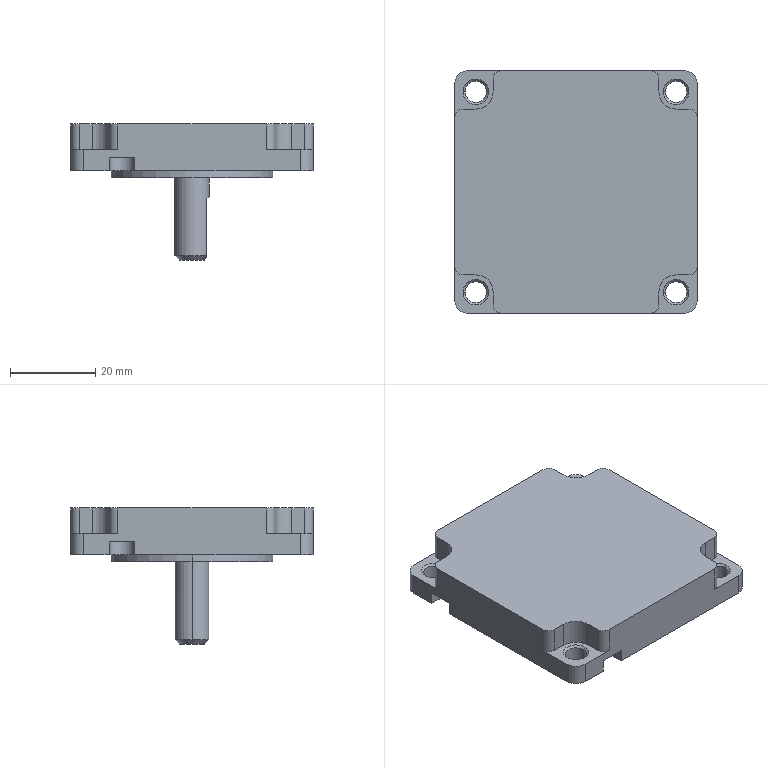Part | SolidWorks | features BaseBody 1 | 1 solid | 86 faces | box 57 x 57 x 32 mm | volume 35610 mm3 | cylinder 39 | plane 37 | cone 10 | commonest cylinder face diameters 6 x9 4 x8 5 x8 8 x8 10 x4 38.1 x2